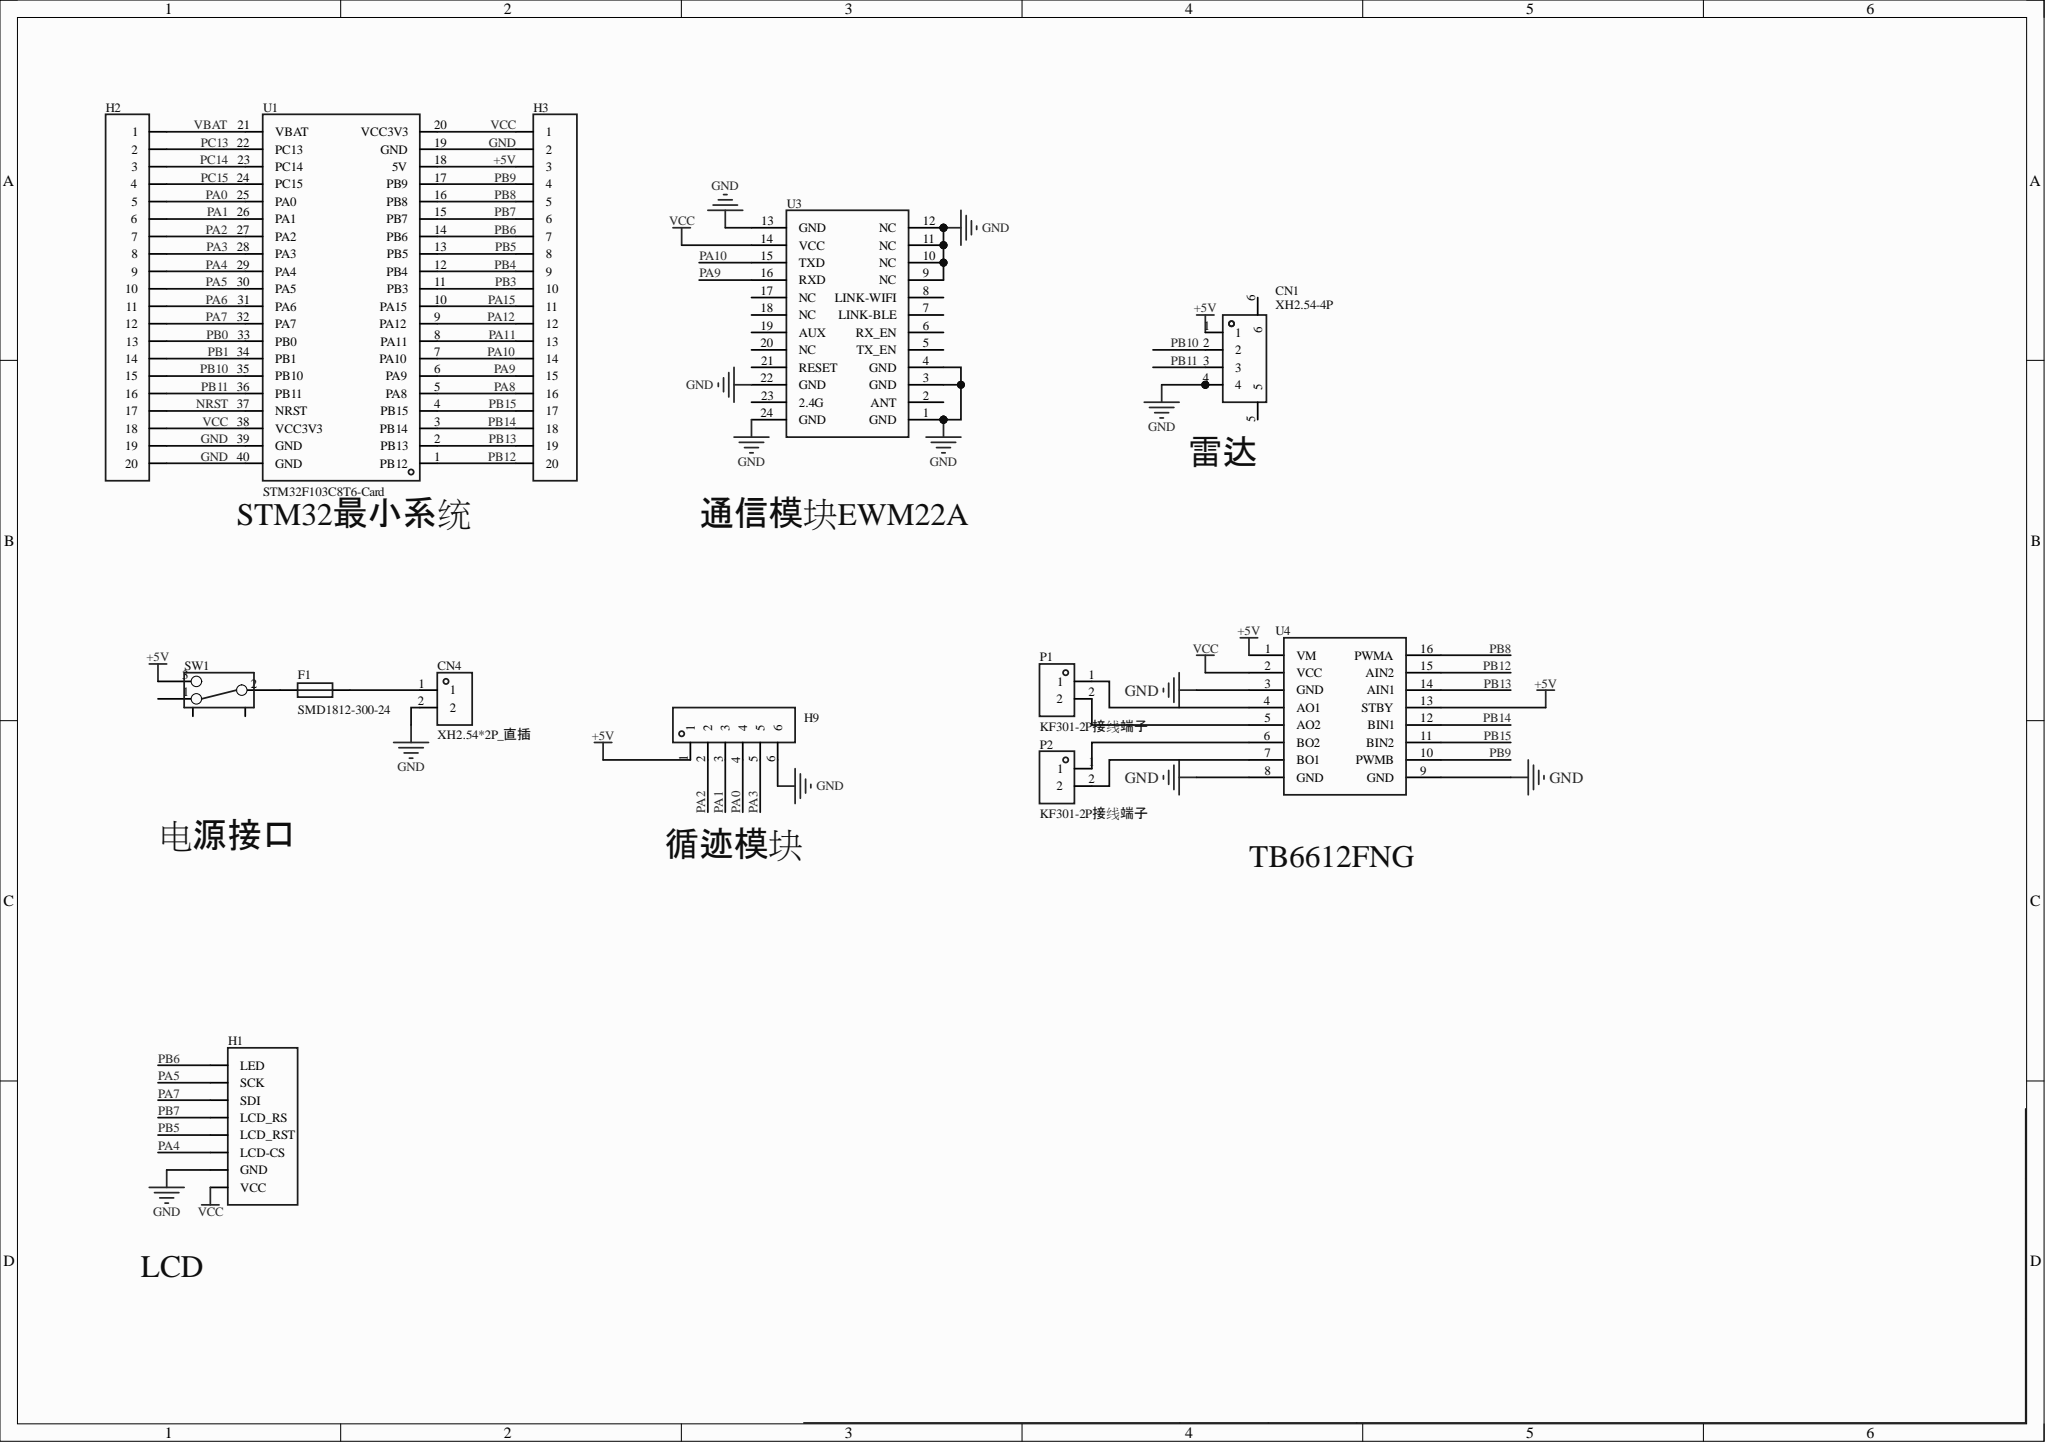Circuit board | Altium Designer | 13 parts | 43 nets
Bill of materials:
Comment,Description,Designator,Footprint,LibRef,Quantity
"XH2.54-4P","","CN1","CONN-SMD_4P-P2.50-WT","XH2.54-4P","1"
"XH2.54*2P_直插","","CN4","CONN-TH_2P-P2.50-XH2.54-2P","XH2.54*2P_直插","1"
"SMD1812-300-24","耐压(Vmax):24V;最大电流(Imax):40A;保持电流(Ihold):3A;跳闸电流(Itrip):6A;","F1","F1812","SMD1812-300-24","1"
"","","H1","HDR-TH_8P-P2.54-V-F-1","HDR-F_2.54_1x8P","1"
"","","H2, H3","HDR-TH_20P-P2.54-V-F","HDR-F_2.54_1x20P","2"
"","","H9","HDR-TH_6P-P2.54-V-F","HDR-F_2.54_1x6P","1"
"KF301-2P接线端子","","P1, P2","CONN-TH_XY301V-A-5.0-2P","KF301-2P接线端子","2"
"","","SW1","拨动开关_侧","拨动开关_侧","1"
"STM32F103C8T6-Card","","U1","CONN-TH_L53.3-W22.9_STM32F103C8T6-CARD","STM32F103C8T6-Card","1"
"","EWM22A-400BWL22S","U3","EWM22M-400/900T22S","EWM22A-400BWL22S","1"
"","","U4","tb6612","tb6612","1"
Netlist (Protel format):
[
CN1
CONN-SMD_4P-P2.50-WT
XH2.54-4P



]
[
CN4
CONN-TH_2P-P2.50-XH2.54-2P
XH2.54*2P_直插



]
[
F1
F1812
SMD1812-300-24



]
[
H1
HDR-TH_8P-P2.54-V-F-1




]
[
H2
HDR-TH_20P-P2.54-V-F




]
[
H3
HDR-TH_20P-P2.54-V-F




]
[
H9
HDR-TH_6P-P2.54-V-F




]
[
P1
CONN-TH_XY301V-A-5.0-2P
KF301-2P接线端子



]
[
P2
CONN-TH_XY301V-A-5.0-2P
KF301-2P接线端子



]
[
SW1
拨动开关_侧




]
[
U1
CONN-TH_L53.3-W22.9_STM32F103C8T6-CARD
STM32F103C8T6-Card



]
[
U3
EWM22M-400/900T22S




]
[
U4
tb6612




]
(
VCC
H1-8
H2-18
H3-1
U1-20
U1-38
U3-14
U4-2
)
(
VBAT
H2-1
U1-21
)
(
PC15
H2-4
U1-24
)
(
PC14
H2-3
U1-23
)
(
PC13
H2-2
U1-22
)
(
PB15
H3-17
U1-4
U4-11
)
(
PB14
H3-18
U1-3
U4-12
)
(
PB13
H3-19
U1-2
U4-14
)
(
PB12
H3-20
U1-1
U4-15
)
(
PB11
CN1-3
H2-16
U1-36
)
(
PB10
CN1-2
H2-15
U1-35
)
(
PB9
H3-4
U1-17
U4-10
)
(
PB8
H3-5
U1-16
U4-16
)
(
PB7
H1-4
H3-6
U1-15
)
(
PB6
H1-1
H3-7
U1-14
)
(
PB5
H1-5
H3-8
U1-13
)
(
PB4
H3-9
U1-12
)
(
PB3
H3-10
U1-11
)
(
PB1
H2-14
U1-34
)
(
PB0
H2-13
U1-33
)
(
PA15
H3-11
U1-10
)
(
PA12
H3-12
U1-9
)
(
PA11
H3-13
U1-8
)
(
PA10
H3-14
U1-7
U3-15
)
(
PA9
H3-15
U1-6
U3-16
)
(
PA8
H3-16
U1-5
)
(
PA7
H1-3
H2-12
U1-32
)
(
PA6
H2-11
U1-31
)
(
PA5
H1-2
H2-10
U1-30
)
(
PA4
H1-6
H2-9
U1-29
)
(
PA3
H2-8
H9-5
U1-28
)
(
PA2
H2-7
H9-2
U1-27
)
(
PA1
H2-6
H9-3
U1-26
)
(
PA0
H2-5
H9-4
U1-25
)
(
NRST
H2-17
U1-37
)
(
NetP2_2
P2-2
U4-7
)
(
NetP2_1
P2-1
U4-6
)
(
NetP1_2
P1-2
U4-5
)
(
NetP1_1
P1-1
U4-4
)
(
NetF1_1
F1-1
SW1-2
)
(
NetCN4_1
CN4-1
F1-2
)
(
GND
CN1-4
CN4-2
H1-7
H2-19
H2-20
H3-2
H9-6
U1-19
U1-39
U1-40
U3-1
U3-3
U3-4
U3-9
U3-10
U3-11
U3-12
U3-13
U3-22
U3-24
U4-3
U4-8
U4-9
)
(
+5V
CN1-1
H3-3
H9-1
SW1-3
U1-18
U4-1
U4-13
)